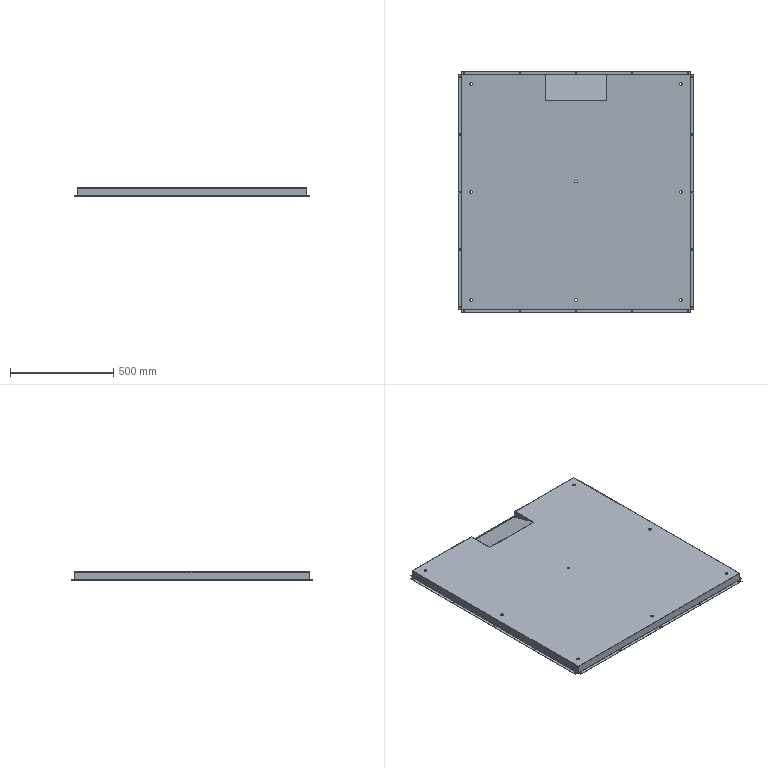Part | 2 solids | 206 faces | box 1139 x 1169 x 40 mm | volume 1495333 mm3 | plane 106 | cylinder 88 | spline 12 | commonest cylinder face diameters 7 x50 14 x14 0.4 x11 2.4 x11 11 x2